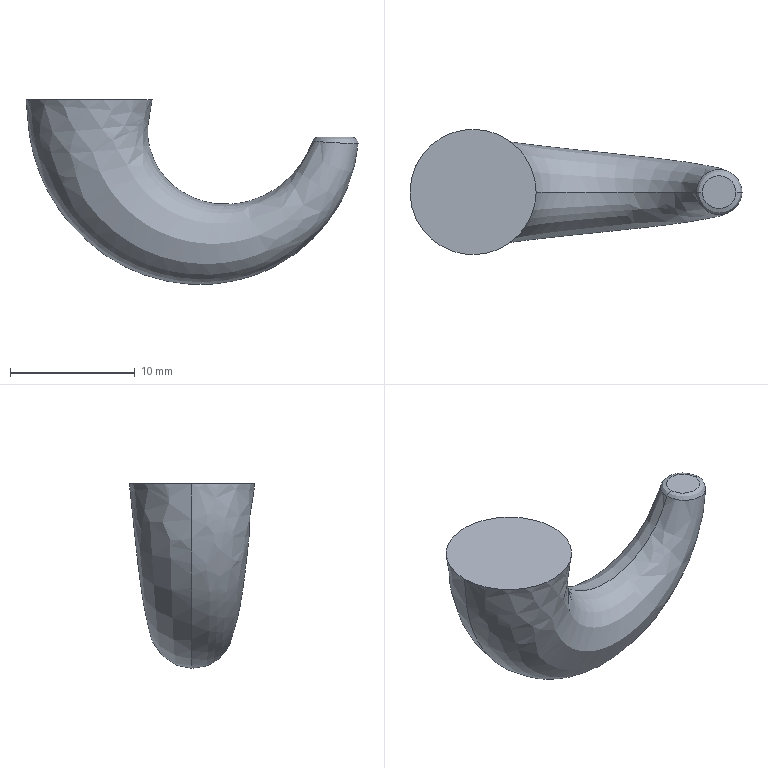Part | STEP file | solid 211 | 1 solid | 6 faces | box 26.578 x 10.027 x 14.799 mm | volume 1219 mm3 | spline 4 | plane 2